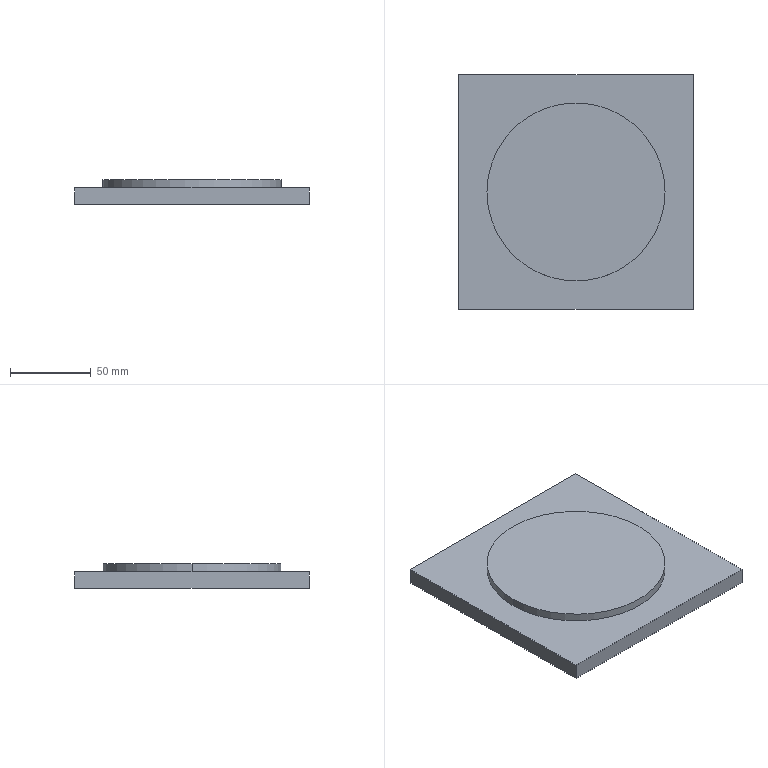Part | SolidWorks | features Extrusion 1, ICE 1 | 1 solid | 9 faces | box 145 x 145 x 15 mm | volume 257767 mm3 | plane 7 | cylinder 2 | commonest cylinder face diameters 110 x2
STEP:
#1=CARTESIAN_POINT('',(127.5,72.5,15.));
#2=VERTEX_POINT('',#1);
#3=CARTESIAN_POINT('',(17.5,72.5,15.));
#4=VERTEX_POINT('',#3);
#5=CARTESIAN_POINT('',(72.5,72.5,15.));
#6=DIRECTION('',(0.,0.,1.));
#7=DIRECTION('',(1.,0.,0.));
#8=AXIS2_PLACEMENT_3D('',#5,#6,#7);
#9=CIRCLE('',#8,55.);
#10=EDGE_CURVE('',#2,#4,#9,.T.);
#11=ORIENTED_EDGE('',*,*,#10,.F.);
#12=CARTESIAN_POINT('',(127.5,72.5,10.));
#13=VERTEX_POINT('',#12);
#14=CARTESIAN_POINT('',(127.5,72.5,15.));
#15=DIRECTION('',(0.,0.,-1.));
#16=VECTOR('',#15,1000.);
#17=LINE('',#14,#16);
#18=EDGE_CURVE('',#2,#13,#17,.T.);
#19=ORIENTED_EDGE('',*,*,#18,.T.);
#20=CARTESIAN_POINT('',(17.5,72.5,10.));
#21=VERTEX_POINT('',#20);
#22=CARTESIAN_POINT('',(72.5,72.5,10.));
#23=DIRECTION('',(0.,0.,1.));
#24=DIRECTION('',(-1.,0.,0.));
#25=AXIS2_PLACEMENT_3D('',#22,#23,#24);
#26=CIRCLE('',#25,55.);
#27=EDGE_CURVE('',#13,#21,#26,.T.);
#28=ORIENTED_EDGE('',*,*,#27,.T.);
#29=CARTESIAN_POINT('',(17.5,72.5,15.));
#30=DIRECTION('',(0.,0.,-1.));
#31=VECTOR('',#30,1000.);
#32=LINE('',#29,#31);
#33=EDGE_CURVE('',#4,#21,#32,.T.);
#34=ORIENTED_EDGE('',*,*,#33,.F.);
#35=EDGE_LOOP('',(#11,#19,#28,#34));
#36=FACE_OUTER_BOUND('',#35,.T.);
#37=CARTESIAN_POINT('',(72.5,72.5,15.));
#38=DIRECTION('',(0.,0.,-1.));
#39=DIRECTION('',(-1.,0.,0.));
#40=AXIS2_PLACEMENT_3D('',#37,#38,#39);
#41=CYLINDRICAL_SURFACE('',#40,55.);
#42=ADVANCED_FACE('',(#36),#41,.T.);
#43=CARTESIAN_POINT('',(0.,145.,10.));
#44=VERTEX_POINT('',#43);
#45=CARTESIAN_POINT('',(0.,0.,10.));
#46=VERTEX_POINT('',#45);
#47=CARTESIAN_POINT('',(0.,0.,10.));
#48=DIRECTION('',(0.,-1.,0.));
#49=VECTOR('',#48,1000.);
#50=LINE('',#47,#49);
#51=EDGE_CURVE('',#44,#46,#50,.T.);
#52=ORIENTED_EDGE('',*,*,#51,.T.);
#53=CARTESIAN_POINT('',(145.,0.,10.));
#54=VERTEX_POINT('',#53);
#55=CARTESIAN_POINT('',(0.,0.,10.));
#56=DIRECTION('',(1.,0.,0.));
#57=VECTOR('',#56,1000.);
#58=LINE('',#55,#57);
#59=EDGE_CURVE('',#46,#54,#58,.T.);
#60=ORIENTED_EDGE('',*,*,#59,.T.);
#61=CARTESIAN_POINT('',(145.,145.,10.));
#62=VERTEX_POINT('',#61);
#63=CARTESIAN_POINT('',(145.,145.,10.));
#64=DIRECTION('',(0.,1.,0.));
#65=VECTOR('',#64,1000.);
#66=LINE('',#63,#65);
#67=EDGE_CURVE('',#54,#62,#66,.T.);
#68=ORIENTED_EDGE('',*,*,#67,.T.);
#69=CARTESIAN_POINT('',(0.,145.,10.));
#70=DIRECTION('',(-1.,0.,0.));
#71=VECTOR('',#70,1000.);
#72=LINE('',#69,#71);
#73=EDGE_CURVE('',#62,#44,#72,.T.);
#74=ORIENTED_EDGE('',*,*,#73,.T.);
#75=EDGE_LOOP('',(#52,#60,#68,#74));
#76=FACE_OUTER_BOUND('',#75,.T.);
#77=CARTESIAN_POINT('',(72.5,72.5,10.));
#78=DIRECTION('',(0.,0.,1.));
#79=DIRECTION('',(-1.,0.,0.));
#80=AXIS2_PLACEMENT_3D('',#77,#78,#79);
#81=CIRCLE('',#80,55.);
#82=EDGE_CURVE('',#21,#13,#81,.T.);
#83=ORIENTED_EDGE('',*,*,#82,.F.);
#84=ORIENTED_EDGE('',*,*,#27,.F.);
#85=EDGE_LOOP('',(#83,#84));
#86=FACE_BOUND('',#85,.T.);
#87=CARTESIAN_POINT('',(0.,145.,10.));
#88=DIRECTION('',(0.,0.,-1.));
#89=DIRECTION('',(-1.,0.,0.));
#90=AXIS2_PLACEMENT_3D('',#87,#88,#89);
#91=PLANE('',#90);
#92=ADVANCED_FACE('',(#76,#86),#91,.F.);
#93=CARTESIAN_POINT('',(0.,145.,0.));
#94=VERTEX_POINT('',#93);
#95=CARTESIAN_POINT('',(0.,0.,0.));
#96=VERTEX_POINT('',#95);
#97=CARTESIAN_POINT('',(0.,0.,0.));
#98=DIRECTION('',(0.,-1.,0.));
#99=VECTOR('',#98,1000.);
#100=LINE('',#97,#99);
#101=EDGE_CURVE('',#94,#96,#100,.T.);
#102=ORIENTED_EDGE('',*,*,#101,.T.);
#103=CARTESIAN_POINT('',(0.,0.,10.));
#104=DIRECTION('',(0.,0.,-1.));
#105=VECTOR('',#104,1000.);
#106=LINE('',#103,#105);
#107=EDGE_CURVE('',#46,#96,#106,.T.);
#108=ORIENTED_EDGE('',*,*,#107,.F.);
#109=ORIENTED_EDGE('',*,*,#51,.F.);
#110=CARTESIAN_POINT('',(0.,145.,10.));
#111=DIRECTION('',(0.,0.,-1.));
#112=VECTOR('',#111,1000.);
#113=LINE('',#110,#112);
#114=EDGE_CURVE('',#44,#94,#113,.T.);
#115=ORIENTED_EDGE('',*,*,#114,.T.);
#116=EDGE_LOOP('',(#102,#108,#109,#115));
#117=FACE_OUTER_BOUND('',#116,.T.);
#118=CARTESIAN_POINT('',(0.,0.,10.));
#119=DIRECTION('',(1.,0.,0.));
#120=DIRECTION('',(0.,0.,-1.));
#121=AXIS2_PLACEMENT_3D('',#118,#119,#120);
#122=PLANE('',#121);
#123=ADVANCED_FACE('',(#117),#122,.F.);
#124=CARTESIAN_POINT('',(145.,0.,0.));
#125=VERTEX_POINT('',#124);
#126=CARTESIAN_POINT('',(0.,0.,0.));
#127=DIRECTION('',(1.,0.,0.));
#128=VECTOR('',#127,1000.);
#129=LINE('',#126,#128);
#130=EDGE_CURVE('',#96,#125,#129,.T.);
#131=ORIENTED_EDGE('',*,*,#130,.T.);
#132=CARTESIAN_POINT('',(145.,0.,10.));
#133=DIRECTION('',(0.,0.,-1.));
#134=VECTOR('',#133,1000.);
#135=LINE('',#132,#134);
#136=EDGE_CURVE('',#54,#125,#135,.T.);
#137=ORIENTED_EDGE('',*,*,#136,.F.);
#138=ORIENTED_EDGE('',*,*,#59,.F.);
#139=ORIENTED_EDGE('',*,*,#107,.T.);
#140=EDGE_LOOP('',(#131,#137,#138,#139));
#141=FACE_OUTER_BOUND('',#140,.T.);
#142=CARTESIAN_POINT('',(0.,0.,10.));
#143=DIRECTION('',(0.,1.,0.));
#144=DIRECTION('',(0.,0.,1.));
#145=AXIS2_PLACEMENT_3D('',#142,#143,#144);
#146=PLANE('',#145);
#147=ADVANCED_FACE('',(#141),#146,.F.);
#148=CARTESIAN_POINT('',(145.,145.,0.));
#149=VERTEX_POINT('',#148);
#150=CARTESIAN_POINT('',(145.,145.,0.));
#151=DIRECTION('',(0.,1.,0.));
#152=VECTOR('',#151,1000.);
#153=LINE('',#150,#152);
#154=EDGE_CURVE('',#125,#149,#153,.T.);
#155=ORIENTED_EDGE('',*,*,#154,.T.);
#156=CARTESIAN_POINT('',(145.,145.,10.));
#157=DIRECTION('',(0.,0.,-1.));
#158=VECTOR('',#157,1000.);
#159=LINE('',#156,#158);
#160=EDGE_CURVE('',#62,#149,#159,.T.);
#161=ORIENTED_EDGE('',*,*,#160,.F.);
#162=ORIENTED_EDGE('',*,*,#67,.F.);
#163=ORIENTED_EDGE('',*,*,#136,.T.);
#164=EDGE_LOOP('',(#155,#161,#162,#163));
#165=FACE_OUTER_BOUND('',#164,.T.);
#166=CARTESIAN_POINT('',(145.,145.,10.));
#167=DIRECTION('',(-1.,0.,0.));
#168=DIRECTION('',(0.,-1.,0.));
#169=AXIS2_PLACEMENT_3D('',#166,#167,#168);
#170=PLANE('',#169);
#171=ADVANCED_FACE('',(#165),#170,.F.);
#172=CARTESIAN_POINT('',(0.,145.,0.));
#173=DIRECTION('',(-1.,0.,0.));
#174=VECTOR('',#173,1000.);
#175=LINE('',#172,#174);
#176=EDGE_CURVE('',#149,#94,#175,.T.);
#177=ORIENTED_EDGE('',*,*,#176,.T.);
#178=ORIENTED_EDGE('',*,*,#114,.F.);
#179=ORIENTED_EDGE('',*,*,#73,.F.);
#180=ORIENTED_EDGE('',*,*,#160,.T.);
#181=EDGE_LOOP('',(#177,#178,#179,#180));
#182=FACE_OUTER_BOUND('',#181,.T.);
#183=CARTESIAN_POINT('',(0.,145.,10.));
#184=DIRECTION('',(0.,-1.,0.));
#185=DIRECTION('',(0.,0.,-1.));
#186=AXIS2_PLACEMENT_3D('',#183,#184,#185);
#187=PLANE('',#186);
#188=ADVANCED_FACE('',(#182),#187,.F.);
#189=ORIENTED_EDGE('',*,*,#101,.F.);
#190=ORIENTED_EDGE('',*,*,#176,.F.);
#191=ORIENTED_EDGE('',*,*,#154,.F.);
#192=ORIENTED_EDGE('',*,*,#130,.F.);
#193=EDGE_LOOP('',(#189,#190,#191,#192));
#194=FACE_OUTER_BOUND('',#193,.T.);
#195=CARTESIAN_POINT('',(0.,145.,0.));
#196=DIRECTION('',(0.,0.,-1.));
#197=DIRECTION('',(-1.,0.,0.));
#198=AXIS2_PLACEMENT_3D('',#195,#196,#197);
#199=PLANE('',#198);
#200=ADVANCED_FACE('',(#194),#199,.T.);
#201=ORIENTED_EDGE('',*,*,#18,.F.);
#202=CARTESIAN_POINT('',(72.5,72.5,15.));
#203=DIRECTION('',(0.,0.,1.));
#204=DIRECTION('',(1.,0.,0.));
#205=AXIS2_PLACEMENT_3D('',#202,#203,#204);
#206=CIRCLE('',#205,55.);
#207=EDGE_CURVE('',#4,#2,#206,.T.);
#208=ORIENTED_EDGE('',*,*,#207,.F.);
#209=ORIENTED_EDGE('',*,*,#33,.T.);
#210=ORIENTED_EDGE('',*,*,#82,.T.);
#211=EDGE_LOOP('',(#201,#208,#209,#210));
#212=FACE_OUTER_BOUND('',#211,.T.);
#213=CARTESIAN_POINT('',(72.5,72.5,15.));
#214=DIRECTION('',(0.,0.,-1.));
#215=DIRECTION('',(-1.,0.,0.));
#216=AXIS2_PLACEMENT_3D('',#213,#214,#215);
#217=CYLINDRICAL_SURFACE('',#216,55.);
#218=ADVANCED_FACE('',(#212),#217,.T.);
#219=ORIENTED_EDGE('',*,*,#207,.T.);
#220=ORIENTED_EDGE('',*,*,#10,.T.);
#221=EDGE_LOOP('',(#219,#220));
#222=FACE_OUTER_BOUND('',#221,.T.);
#223=CARTESIAN_POINT('',(72.5,72.5,15.));
#224=DIRECTION('',(0.,0.,1.));
#225=DIRECTION('',(1.,0.,0.));
#226=AXIS2_PLACEMENT_3D('',#223,#224,#225);
#227=PLANE('',#226);
#228=ADVANCED_FACE('',(#222),#227,.T.);
#229=CLOSED_SHELL('',(#42,#92,#123,#147,#171,#188,#200,#218,#228));
#230=MANIFOLD_SOLID_BREP('',#229);
#231=CARTESIAN_POINT('',(0.,0.,0.));
#232=DIRECTION('',(0.,0.,1.));
#233=DIRECTION('',(1.,0.,0.));
#234=AXIS2_PLACEMENT_3D('',#231,#232,#233);
#235=(LENGTH_UNIT()NAMED_UNIT(*)SI_UNIT(.MILLI.,.METRE.));
#236=UNCERTAINTY_MEASURE_WITH_UNIT(LENGTH_MEASURE(0.00001),#235,'','');
#237=(NAMED_UNIT(*)PLANE_ANGLE_UNIT()SI_UNIT($,.RADIAN.));
#238=(NAMED_UNIT(*)SI_UNIT($,.STERADIAN.)SOLID_ANGLE_UNIT());
#239=(GEOMETRIC_REPRESENTATION_CONTEXT(3)GLOBAL_UNCERTAINTY_ASSIGNED_CONTEXT((#236))GLOBAL_UNIT_ASSIGNED_CONTEXT((#235,#237,#238))REPRESENTATION_CONTEXT('',''));
#240=ADVANCED_BREP_SHAPE_REPRESENTATION('',(#230,#234),#239);